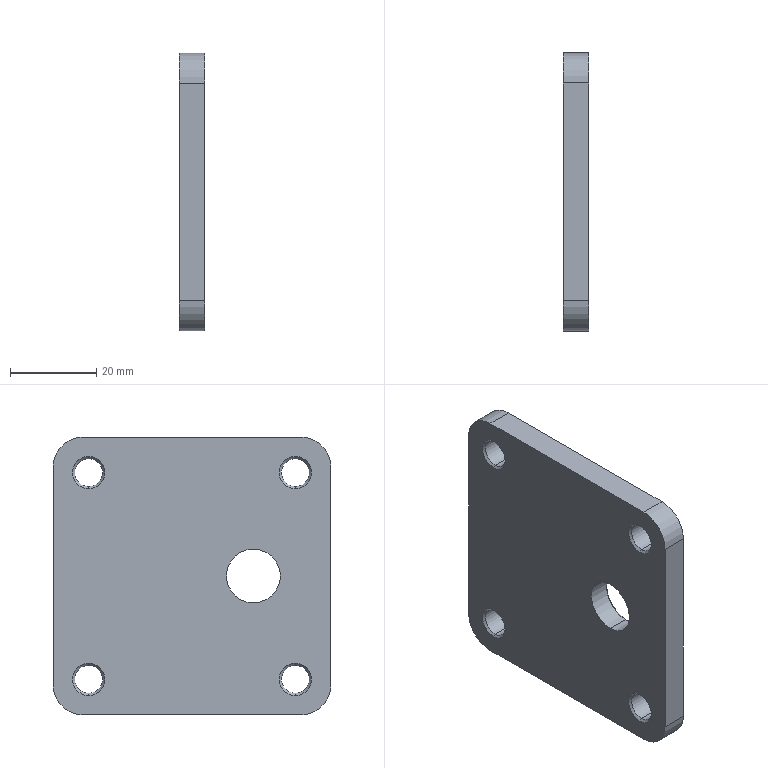Part | SolidWorks | features BaseBody 1 | 1 solid | 41 faces | box 6 x 64.5 x 64.5 mm | volume 23021 mm3 | cone 18 | cylinder 16 | plane 7 | commonest cylinder face diameters 6.5 x8 14 x4 12.5 x2 22 x2
STEP:
#1=CARTESIAN_POINT('',(443.9,24.75,6.25));
#2=VERTEX_POINT('',#1);
#3=CARTESIAN_POINT('',(443.9,24.75,-6.25));
#4=VERTEX_POINT('',#3);
#5=CARTESIAN_POINT('',(443.9,24.75,0.));
#6=DIRECTION('',(1.,0.,0.));
#7=DIRECTION('',(0.,0.,1.));
#8=AXIS2_PLACEMENT_3D('',#5,#6,#7);
#9=CIRCLE('',#8,6.25);
#10=EDGE_CURVE('',#2,#4,#9,.T.);
#11=ORIENTED_EDGE('',*,*,#10,.F.);
#12=CARTESIAN_POINT('',(444.4,24.75,6.75));
#13=VERTEX_POINT('',#12);
#14=CARTESIAN_POINT('',(443.9,24.75,6.25));
#15=DIRECTION('',(0.7071,0.,0.7071));
#16=VECTOR('',#15,1000.);
#17=LINE('',#14,#16);
#18=EDGE_CURVE('',#2,#13,#17,.T.);
#19=ORIENTED_EDGE('',*,*,#18,.T.);
#20=CARTESIAN_POINT('',(444.4,24.75,-6.75));
#21=VERTEX_POINT('',#20);
#22=CARTESIAN_POINT('',(444.4,24.75,0.));
#23=DIRECTION('',(-1.,0.,0.));
#24=DIRECTION('',(0.,0.,1.));
#25=AXIS2_PLACEMENT_3D('',#22,#23,#24);
#26=CIRCLE('',#25,6.75);
#27=EDGE_CURVE('',#21,#13,#26,.T.);
#28=ORIENTED_EDGE('',*,*,#27,.F.);
#29=CARTESIAN_POINT('',(443.9,24.75,-6.25));
#30=DIRECTION('',(0.7071,0.,-0.7071));
#31=VECTOR('',#30,1000.);
#32=LINE('',#29,#31);
#33=EDGE_CURVE('',#4,#21,#32,.T.);
#34=ORIENTED_EDGE('',*,*,#33,.F.);
#35=EDGE_LOOP('',(#11,#19,#28,#34));
#36=FACE_OUTER_BOUND('',#35,.T.);
#37=CARTESIAN_POINT('',(443.9,24.75,0.));
#38=DIRECTION('',(1.,0.,0.));
#39=DIRECTION('',(0.,0.,-1.));
#40=AXIS2_PLACEMENT_3D('',#37,#38,#39);
#41=CONICAL_SURFACE('',#40,6.25,0.7854);
#42=ADVANCED_FACE('',(#36),#41,.F.);
#43=CARTESIAN_POINT('',(444.4,63.,27.25));
#44=VERTEX_POINT('',#43);
#45=CARTESIAN_POINT('',(444.4,63.,20.75));
#46=VERTEX_POINT('',#45);
#47=CARTESIAN_POINT('',(444.4,63.,24.));
#48=DIRECTION('',(1.,0.,0.));
#49=DIRECTION('',(0.,0.,-1.));
#50=AXIS2_PLACEMENT_3D('',#47,#48,#49);
#51=CIRCLE('',#50,3.25);
#52=EDGE_CURVE('',#44,#46,#51,.T.);
#53=ORIENTED_EDGE('',*,*,#52,.F.);
#54=CARTESIAN_POINT('',(444.9,63.,27.75));
#55=VERTEX_POINT('',#54);
#56=CARTESIAN_POINT('',(444.4,63.,27.25));
#57=DIRECTION('',(0.7071,0.,0.7071));
#58=VECTOR('',#57,1000.);
#59=LINE('',#56,#58);
#60=EDGE_CURVE('',#44,#55,#59,.T.);
#61=ORIENTED_EDGE('',*,*,#60,.T.);
#62=CARTESIAN_POINT('',(444.9,63.,20.25));
#63=VERTEX_POINT('',#62);
#64=CARTESIAN_POINT('',(444.9,63.,24.));
#65=DIRECTION('',(-1.,0.,0.));
#66=DIRECTION('',(0.,0.,-1.));
#67=AXIS2_PLACEMENT_3D('',#64,#65,#66);
#68=CIRCLE('',#67,3.75);
#69=EDGE_CURVE('',#63,#55,#68,.T.);
#70=ORIENTED_EDGE('',*,*,#69,.F.);
#71=CARTESIAN_POINT('',(444.4,63.,20.75));
#72=DIRECTION('',(0.7071,0.,-0.7071));
#73=VECTOR('',#72,1000.);
#74=LINE('',#71,#73);
#75=EDGE_CURVE('',#46,#63,#74,.T.);
#76=ORIENTED_EDGE('',*,*,#75,.F.);
#77=EDGE_LOOP('',(#53,#61,#70,#76));
#78=FACE_OUTER_BOUND('',#77,.T.);
#79=CARTESIAN_POINT('',(444.4,63.,24.));
#80=DIRECTION('',(1.,0.,0.));
#81=DIRECTION('',(0.,0.,-1.));
#82=AXIS2_PLACEMENT_3D('',#79,#80,#81);
#83=CONICAL_SURFACE('',#82,3.25,0.7854);
#84=ADVANCED_FACE('',(#78),#83,.F.);
#85=CARTESIAN_POINT('',(444.4,63.,-20.75));
#86=VERTEX_POINT('',#85);
#87=CARTESIAN_POINT('',(444.4,63.,-27.25));
#88=VERTEX_POINT('',#87);
#89=CARTESIAN_POINT('',(444.4,63.,-24.));
#90=DIRECTION('',(1.,0.,0.));
#91=DIRECTION('',(0.,0.,-1.));
#92=AXIS2_PLACEMENT_3D('',#89,#90,#91);
#93=CIRCLE('',#92,3.25);
#94=EDGE_CURVE('',#86,#88,#93,.T.);
#95=ORIENTED_EDGE('',*,*,#94,.F.);
#96=CARTESIAN_POINT('',(444.9,63.,-20.25));
#97=VERTEX_POINT('',#96);
#98=CARTESIAN_POINT('',(444.4,63.,-20.75));
#99=DIRECTION('',(0.7071,0.,0.7071));
#100=VECTOR('',#99,1000.);
#101=LINE('',#98,#100);
#102=EDGE_CURVE('',#86,#97,#101,.T.);
#103=ORIENTED_EDGE('',*,*,#102,.T.);
#104=CARTESIAN_POINT('',(444.9,63.,-27.75));
#105=VERTEX_POINT('',#104);
#106=CARTESIAN_POINT('',(444.9,63.,-24.));
#107=DIRECTION('',(-1.,0.,0.));
#108=DIRECTION('',(0.,0.,-1.));
#109=AXIS2_PLACEMENT_3D('',#106,#107,#108);
#110=CIRCLE('',#109,3.75);
#111=EDGE_CURVE('',#105,#97,#110,.T.);
#112=ORIENTED_EDGE('',*,*,#111,.F.);
#113=CARTESIAN_POINT('',(444.4,63.,-27.25));
#114=DIRECTION('',(0.7071,0.,-0.7071));
#115=VECTOR('',#114,1000.);
#116=LINE('',#113,#115);
#117=EDGE_CURVE('',#88,#105,#116,.T.);
#118=ORIENTED_EDGE('',*,*,#117,.F.);
#119=EDGE_LOOP('',(#95,#103,#112,#118));
#120=FACE_OUTER_BOUND('',#119,.T.);
#121=CARTESIAN_POINT('',(444.4,63.,-24.));
#122=DIRECTION('',(1.,0.,0.));
#123=DIRECTION('',(0.,0.,-1.));
#124=AXIS2_PLACEMENT_3D('',#121,#122,#123);
#125=CONICAL_SURFACE('',#124,3.25,0.7854);
#126=ADVANCED_FACE('',(#120),#125,.F.);
#127=CARTESIAN_POINT('',(444.4,15.,-20.75));
#128=VERTEX_POINT('',#127);
#129=CARTESIAN_POINT('',(444.4,15.,-27.25));
#130=VERTEX_POINT('',#129);
#131=CARTESIAN_POINT('',(444.4,15.,-24.));
#132=DIRECTION('',(1.,0.,0.));
#133=DIRECTION('',(0.,0.,-1.));
#134=AXIS2_PLACEMENT_3D('',#131,#132,#133);
#135=CIRCLE('',#134,3.25);
#136=EDGE_CURVE('',#128,#130,#135,.T.);
#137=ORIENTED_EDGE('',*,*,#136,.F.);
#138=CARTESIAN_POINT('',(444.9,15.,-20.25));
#139=VERTEX_POINT('',#138);
#140=CARTESIAN_POINT('',(444.4,15.,-20.75));
#141=DIRECTION('',(0.7071,0.,0.7071));
#142=VECTOR('',#141,1000.);
#143=LINE('',#140,#142);
#144=EDGE_CURVE('',#128,#139,#143,.T.);
#145=ORIENTED_EDGE('',*,*,#144,.T.);
#146=CARTESIAN_POINT('',(444.9,15.,-27.75));
#147=VERTEX_POINT('',#146);
#148=CARTESIAN_POINT('',(444.9,15.,-24.));
#149=DIRECTION('',(-1.,0.,0.));
#150=DIRECTION('',(0.,0.,-1.));
#151=AXIS2_PLACEMENT_3D('',#148,#149,#150);
#152=CIRCLE('',#151,3.75);
#153=EDGE_CURVE('',#147,#139,#152,.T.);
#154=ORIENTED_EDGE('',*,*,#153,.F.);
#155=CARTESIAN_POINT('',(444.4,15.,-27.25));
#156=DIRECTION('',(0.7071,0.,-0.7071));
#157=VECTOR('',#156,1000.);
#158=LINE('',#155,#157);
#159=EDGE_CURVE('',#130,#147,#158,.T.);
#160=ORIENTED_EDGE('',*,*,#159,.F.);
#161=EDGE_LOOP('',(#137,#145,#154,#160));
#162=FACE_OUTER_BOUND('',#161,.T.);
#163=CARTESIAN_POINT('',(444.4,15.,-24.));
#164=DIRECTION('',(1.,0.,0.));
#165=DIRECTION('',(0.,0.,-1.));
#166=AXIS2_PLACEMENT_3D('',#163,#164,#165);
#167=CONICAL_SURFACE('',#166,3.25,0.7854);
#168=ADVANCED_FACE('',(#162),#167,.F.);
#169=CARTESIAN_POINT('',(444.4,15.,27.25));
#170=VERTEX_POINT('',#169);
#171=CARTESIAN_POINT('',(444.4,15.,20.75));
#172=VERTEX_POINT('',#171);
#173=CARTESIAN_POINT('',(444.4,15.,24.));
#174=DIRECTION('',(1.,0.,0.));
#175=DIRECTION('',(0.,0.,-1.));
#176=AXIS2_PLACEMENT_3D('',#173,#174,#175);
#177=CIRCLE('',#176,3.25);
#178=EDGE_CURVE('',#170,#172,#177,.T.);
#179=ORIENTED_EDGE('',*,*,#178,.F.);
#180=CARTESIAN_POINT('',(444.9,15.,27.75));
#181=VERTEX_POINT('',#180);
#182=CARTESIAN_POINT('',(444.4,15.,27.25));
#183=DIRECTION('',(0.7071,0.,0.7071));
#184=VECTOR('',#183,1000.);
#185=LINE('',#182,#184);
#186=EDGE_CURVE('',#170,#181,#185,.T.);
#187=ORIENTED_EDGE('',*,*,#186,.T.);
#188=CARTESIAN_POINT('',(444.9,15.,20.25));
#189=VERTEX_POINT('',#188);
#190=CARTESIAN_POINT('',(444.9,15.,24.));
#191=DIRECTION('',(-1.,0.,0.));
#192=DIRECTION('',(0.,0.,-1.));
#193=AXIS2_PLACEMENT_3D('',#190,#191,#192);
#194=CIRCLE('',#193,3.75);
#195=EDGE_CURVE('',#189,#181,#194,.T.);
#196=ORIENTED_EDGE('',*,*,#195,.F.);
#197=CARTESIAN_POINT('',(444.4,15.,20.75));
#198=DIRECTION('',(0.7071,0.,-0.7071));
#199=VECTOR('',#198,1000.);
#200=LINE('',#197,#199);
#201=EDGE_CURVE('',#172,#189,#200,.T.);
#202=ORIENTED_EDGE('',*,*,#201,.F.);
#203=EDGE_LOOP('',(#179,#187,#196,#202));
#204=FACE_OUTER_BOUND('',#203,.T.);
#205=CARTESIAN_POINT('',(444.4,15.,24.));
#206=DIRECTION('',(1.,0.,0.));
#207=DIRECTION('',(0.,0.,-1.));
#208=AXIS2_PLACEMENT_3D('',#205,#206,#207);
#209=CONICAL_SURFACE('',#208,3.25,0.7854);
#210=ADVANCED_FACE('',(#204),#209,.F.);
#211=CARTESIAN_POINT('',(439.4,63.,20.75));
#212=VERTEX_POINT('',#211);
#213=CARTESIAN_POINT('',(439.4,63.,27.25));
#214=VERTEX_POINT('',#213);
#215=CARTESIAN_POINT('',(439.4,63.,24.));
#216=DIRECTION('',(-1.,0.,0.));
#217=DIRECTION('',(0.,0.,-1.));
#218=AXIS2_PLACEMENT_3D('',#215,#216,#217);
#219=CIRCLE('',#218,3.25);
#220=EDGE_CURVE('',#212,#214,#219,.T.);
#221=ORIENTED_EDGE('',*,*,#220,.F.);
#222=CARTESIAN_POINT('',(438.9,63.,20.25));
#223=VERTEX_POINT('',#222);
#224=CARTESIAN_POINT('',(438.9,63.,20.25));
#225=DIRECTION('',(-0.7071,0.,-0.7071));
#226=VECTOR('',#225,1000.);
#227=LINE('',#224,#226);
#228=EDGE_CURVE('',#212,#223,#227,.T.);
#229=ORIENTED_EDGE('',*,*,#228,.T.);
#230=CARTESIAN_POINT('',(438.9,63.,27.75));
#231=VERTEX_POINT('',#230);
#232=CARTESIAN_POINT('',(438.9,63.,24.));
#233=DIRECTION('',(1.,0.,0.));
#234=DIRECTION('',(0.,0.,-1.));
#235=AXIS2_PLACEMENT_3D('',#232,#233,#234);
#236=CIRCLE('',#235,3.75);
#237=EDGE_CURVE('',#231,#223,#236,.T.);
#238=ORIENTED_EDGE('',*,*,#237,.F.);
#239=CARTESIAN_POINT('',(438.9,63.,27.75));
#240=DIRECTION('',(-0.7071,0.,0.7071));
#241=VECTOR('',#240,1000.);
#242=LINE('',#239,#241);
#243=EDGE_CURVE('',#214,#231,#242,.T.);
#244=ORIENTED_EDGE('',*,*,#243,.F.);
#245=EDGE_LOOP('',(#221,#229,#238,#244));
#246=FACE_OUTER_BOUND('',#245,.T.);
#247=CARTESIAN_POINT('',(438.9,63.,24.));
#248=DIRECTION('',(-1.,0.,0.));
#249=DIRECTION('',(0.,0.,1.));
#250=AXIS2_PLACEMENT_3D('',#247,#248,#249);
#251=CONICAL_SURFACE('',#250,3.75,0.7854);
#252=ADVANCED_FACE('',(#246),#251,.F.);
#253=CARTESIAN_POINT('',(439.4,15.,20.75));
#254=VERTEX_POINT('',#253);
#255=CARTESIAN_POINT('',(439.4,15.,27.25));
#256=VERTEX_POINT('',#255);
#257=CARTESIAN_POINT('',(439.4,15.,24.));
#258=DIRECTION('',(-1.,0.,0.));
#259=DIRECTION('',(0.,0.,-1.));
#260=AXIS2_PLACEMENT_3D('',#257,#258,#259);
#261=CIRCLE('',#260,3.25);
#262=EDGE_CURVE('',#254,#256,#261,.T.);
#263=ORIENTED_EDGE('',*,*,#262,.F.);
#264=CARTESIAN_POINT('',(438.9,15.,20.25));
#265=VERTEX_POINT('',#264);
#266=CARTESIAN_POINT('',(438.9,15.,20.25));
#267=DIRECTION('',(-0.7071,0.,-0.7071));
#268=VECTOR('',#267,1000.);
#269=LINE('',#266,#268);
#270=EDGE_CURVE('',#254,#265,#269,.T.);
#271=ORIENTED_EDGE('',*,*,#270,.T.);
#272=CARTESIAN_POINT('',(438.9,15.,27.75));
#273=VERTEX_POINT('',#272);
#274=CARTESIAN_POINT('',(438.9,15.,24.));
#275=DIRECTION('',(1.,0.,0.));
#276=DIRECTION('',(0.,0.,-1.));
#277=AXIS2_PLACEMENT_3D('',#274,#275,#276);
#278=CIRCLE('',#277,3.75);
#279=EDGE_CURVE('',#273,#265,#278,.T.);
#280=ORIENTED_EDGE('',*,*,#279,.F.);
#281=CARTESIAN_POINT('',(438.9,15.,27.75));
#282=DIRECTION('',(-0.7071,0.,0.7071));
#283=VECTOR('',#282,1000.);
#284=LINE('',#281,#283);
#285=EDGE_CURVE('',#256,#273,#284,.T.);
#286=ORIENTED_EDGE('',*,*,#285,.F.);
#287=EDGE_LOOP('',(#263,#271,#280,#286));
#288=FACE_OUTER_BOUND('',#287,.T.);
#289=CARTESIAN_POINT('',(438.9,15.,24.));
#290=DIRECTION('',(-1.,0.,0.));
#291=DIRECTION('',(0.,0.,1.));
#292=AXIS2_PLACEMENT_3D('',#289,#290,#291);
#293=CONICAL_SURFACE('',#292,3.75,0.7854);
#294=ADVANCED_FACE('',(#288),#293,.F.);
#295=CARTESIAN_POINT('',(439.4,15.,-27.25));
#296=VERTEX_POINT('',#295);
#297=CARTESIAN_POINT('',(439.4,15.,-20.75));
#298=VERTEX_POINT('',#297);
#299=CARTESIAN_POINT('',(439.4,15.,-24.));
#300=DIRECTION('',(-1.,0.,0.));
#301=DIRECTION('',(0.,0.,-1.));
#302=AXIS2_PLACEMENT_3D('',#299,#300,#301);
#303=CIRCLE('',#302,3.25);
#304=EDGE_CURVE('',#296,#298,#303,.T.);
#305=ORIENTED_EDGE('',*,*,#304,.F.);
#306=CARTESIAN_POINT('',(438.9,15.,-27.75));
#307=VERTEX_POINT('',#306);
#308=CARTESIAN_POINT('',(438.9,15.,-27.75));
#309=DIRECTION('',(-0.7071,0.,-0.7071));
#310=VECTOR('',#309,1000.);
#311=LINE('',#308,#310);
#312=EDGE_CURVE('',#296,#307,#311,.T.);
#313=ORIENTED_EDGE('',*,*,#312,.T.);
#314=CARTESIAN_POINT('',(438.9,15.,-20.25));
#315=VERTEX_POINT('',#314);
#316=CARTESIAN_POINT('',(438.9,15.,-24.));
#317=DIRECTION('',(1.,0.,0.));
#318=DIRECTION('',(0.,0.,-1.));
#319=AXIS2_PLACEMENT_3D('',#316,#317,#318);
#320=CIRCLE('',#319,3.75);
#321=EDGE_CURVE('',#315,#307,#320,.T.);
#322=ORIENTED_EDGE('',*,*,#321,.F.);
#323=CARTESIAN_POINT('',(438.9,15.,-20.25));
#324=DIRECTION('',(-0.7071,0.,0.7071));
#325=VECTOR('',#324,1000.);
#326=LINE('',#323,#325);
#327=EDGE_CURVE('',#298,#315,#326,.T.);
#328=ORIENTED_EDGE('',*,*,#327,.F.);
#329=EDGE_LOOP('',(#305,#313,#322,#328));
#330=FACE_OUTER_BOUND('',#329,.T.);
#331=CARTESIAN_POINT('',(438.9,15.,-24.));
#332=DIRECTION('',(-1.,0.,0.));
#333=DIRECTION('',(0.,0.,1.));
#334=AXIS2_PLACEMENT_3D('',#331,#332,#333);
#335=CONICAL_SURFACE('',#334,3.75,0.7854);
#336=ADVANCED_FACE('',(#330),#335,.F.);
#337=CARTESIAN_POINT('',(439.4,63.,-27.25));
#338=VERTEX_POINT('',#337);
#339=CARTESIAN_POINT('',(439.4,63.,-20.75));
#340=VERTEX_POINT('',#339);
#341=CARTESIAN_POINT('',(439.4,63.,-24.));
#342=DIRECTION('',(-1.,0.,0.));
#343=DIRECTION('',(0.,0.,-1.));
#344=AXIS2_PLACEMENT_3D('',#341,#342,#343);
#345=CIRCLE('',#344,3.25);
#346=EDGE_CURVE('',#338,#340,#345,.T.);
#347=ORIENTED_EDGE('',*,*,#346,.F.);
#348=CARTESIAN_POINT('',(438.9,63.,-27.75));
#349=VERTEX_POINT('',#348);
#350=CARTESIAN_POINT('',(438.9,63.,-27.75));
#351=DIRECTION('',(-0.7071,0.,-0.7071));
#352=VECTOR('',#351,1000.);
#353=LINE('',#350,#352);
#354=EDGE_CURVE('',#338,#349,#353,.T.);
#355=ORIENTED_EDGE('',*,*,#354,.T.);
#356=CARTESIAN_POINT('',(438.9,63.,-20.25));
#357=VERTEX_POINT('',#356);
#358=CARTESIAN_POINT('',(438.9,63.,-24.));
#359=DIRECTION('',(1.,0.,0.));
#360=DIRECTION('',(0.,0.,-1.));
#361=AXIS2_PLACEMENT_3D('',#358,#359,#360);
#362=CIRCLE('',#361,3.75);
#363=EDGE_CURVE('',#357,#349,#362,.T.);
#364=ORIENTED_EDGE('',*,*,#363,.F.);
#365=CARTESIAN_POINT('',(438.9,63.,-20.25));
#366=DIRECTION('',(-0.7071,0.,0.7071));
#367=VECTOR('',#366,1000.);
#368=LINE('',#365,#367);
#369=EDGE_CURVE('',#340,#357,#368,.T.);
#370=ORIENTED_EDGE('',*,*,#369,.F.);
#371=EDGE_LOOP('',(#347,#355,#364,#370));
#372=FACE_OUTER_BOUND('',#371,.T.);
#373=CARTESIAN_POINT('',(438.9,63.,-24.));
#374=DIRECTION('',(-1.,0.,0.));
#375=DIRECTION('',(0.,0.,1.));
#376=AXIS2_PLACEMENT_3D('',#373,#374,#375);
#377=CONICAL_SURFACE('',#376,3.75,0.7854);
#378=ADVANCED_FACE('',(#372),#377,.F.);
#379=CARTESIAN_POINT('',(444.4,24.75,-11.));
#380=VERTEX_POINT('',#379);
#381=CARTESIAN_POINT('',(444.4,24.75,11.));
#382=VERTEX_POINT('',#381);
#383=CARTESIAN_POINT('',(444.4,24.75,0.));
#384=DIRECTION('',(-1.,0.,0.));
#385=DIRECTION('',(0.,0.,1.));
#386=AXIS2_PLACEMENT_3D('',#383,#384,#385);
#387=CIRCLE('',#386,11.);
#388=EDGE_CURVE('',#380,#382,#387,.T.);
#389=ORIENTED_EDGE('',*,*,#388,.T.);
#390=CARTESIAN_POINT('',(444.9,24.75,11.));
#391=VERTEX_POINT('',#390);
#392=CARTESIAN_POINT('',(444.4,24.75,11.));
#393=DIRECTION('',(1.,0.,0.));
#394=VECTOR('',#393,1000.);
#395=LINE('',#392,#394);
#396=EDGE_CURVE('',#382,#391,#395,.T.);
#397=ORIENTED_EDGE('',*,*,#396,.T.);
#398=CARTESIAN_POINT('',(444.9,24.75,-11.));
#399=VERTEX_POINT('',#398);
#400=CARTESIAN_POINT('',(444.9,24.75,0.));
#401=DIRECTION('',(-1.,0.,0.));
#402=DIRECTION('',(0.,0.,1.));
#403=AXIS2_PLACEMENT_3D('',#400,#401,#402);
#404=CIRCLE('',#403,11.);
#405=EDGE_CURVE('',#399,#391,#404,.T.);
#406=ORIENTED_EDGE('',*,*,#405,.F.);
#407=CARTESIAN_POINT('',(444.4,24.75,-11.));
#408=DIRECTION('',(1.,0.,0.));
#409=VECTOR('',#408,1000.);
#410=LINE('',#407,#409);
#411=EDGE_CURVE('',#380,#399,#410,.T.);
#412=ORIENTED_EDGE('',*,*,#411,.F.);
#413=EDGE_LOOP('',(#389,#397,#406,#412));
#414=FACE_OUTER_BOUND('',#413,.T.);
#415=CARTESIAN_POINT('',(444.4,24.75,0.));
#416=DIRECTION('',(1.,0.,0.));
#417=DIRECTION('',(0.,0.,-1.));
#418=AXIS2_PLACEMENT_3D('',#415,#416,#417);
#419=CYLINDRICAL_SURFACE('',#418,11.);
#420=ADVANCED_FACE('',(#414),#419,.F.);
#421=ORIENTED_EDGE('',*,*,#10,.T.);
#422=CARTESIAN_POINT('',(438.9,24.75,-6.25));
#423=VERTEX_POINT('',#422);
#424=CARTESIAN_POINT('',(444.9,24.75,-6.25));
#425=DIRECTION('',(-1.,0.,0.));
#426=VECTOR('',#425,1000.);
#427=LINE('',#424,#426);
#428=EDGE_CURVE('',#4,#423,#427,.T.);
#429=ORIENTED_EDGE('',*,*,#428,.T.);
#430=CARTESIAN_POINT('',(438.9,24.75,6.25));
#431=VERTEX_POINT('',#430);
#432=CARTESIAN_POINT('',(438.9,24.75,0.));
#433=DIRECTION('',(-1.,0.,0.));
#434=DIRECTION('',(0.,0.,1.));
#435=AXIS2_PLACEMENT_3D('',#432,#433,#434);
#436=CIRCLE('',#435,6.25);
#437=EDGE_CURVE('',#423,#431,#436,.T.);
#438=ORIENTED_EDGE('',*,*,#437,.T.);
#439=CARTESIAN_POINT('',(444.9,24.75,6.25));
#440=DIRECTION('',(-1.,0.,0.));
#441=VECTOR('',#440,1000.);
#442=LINE('',#439,#441);
#443=EDGE_CURVE('',#2,#431,#442,.T.);
#444=ORIENTED_EDGE('',*,*,#443,.F.);
#445=EDGE_LOOP('',(#421,#429,#438,#444));
#446=FACE_OUTER_BOUND('',#445,.T.);
#447=CARTESIAN_POINT('',(444.9,24.75,0.));
#448=DIRECTION('',(-1.,0.,0.));
#449=DIRECTION('',(0.,0.,1.));
#450=AXIS2_PLACEMENT_3D('',#447,#448,#449);
#451=CYLINDRICAL_SURFACE('',#450,6.25);
#452=ADVANCED_FACE('',(#446),#451,.F.);
#453=ORIENTED_EDGE('',*,*,#94,.T.);
#454=CARTESIAN_POINT('',(444.9,63.,-27.25));
#455=DIRECTION('',(-1.,0.,0.));
#456=VECTOR('',#455,1000.);
#457=LINE('',#454,#456);
#458=EDGE_CURVE('',#88,#338,#457,.T.);
#459=ORIENTED_EDGE('',*,*,#458,.T.);
#460=ORIENTED_EDGE('',*,*,#346,.T.);
#461=CARTESIAN_POINT('',(444.9,63.,-20.75));
#462=DIRECTION('',(-1.,0.,0.));
#463=VECTOR('',#462,1000.);
#464=LINE('',#461,#463);
#465=EDGE_CURVE('',#86,#340,#464,.T.);
#466=ORIENTED_EDGE('',*,*,#465,.F.);
#467=EDGE_LOOP('',(#453,#459,#460,#466));
#468=FACE_OUTER_BOUND('',#467,.T.);
#469=CARTESIAN_POINT('',(444.9,63.,-24.));
#470=DIRECTION('',(-1.,0.,0.));
#471=DIRECTION('',(0.,0.,1.));
#472=AXIS2_PLACEMENT_3D('',#469,#470,#471);
#473=CYLINDRICAL_SURFACE('',#472,3.25);
#474=ADVANCED_FACE('',(#468),#473,.F.);
#475=ORIENTED_EDGE('',*,*,#52,.T.);
#476=CARTESIAN_POINT('',(444.9,63.,20.75));
#477=DIRECTION('',(-1.,0.,0.));
#478=VECTOR('',#477,1000.);
#479=LINE('',#476,#478);
#480=EDGE_CURVE('',#46,#212,#479,.T.);
#481=ORIENTED_EDGE('',*,*,#480,.T.);
#482=ORIENTED_EDGE('',*,*,#220,.T.);
#483=CARTESIAN_POINT('',(444.9,63.,27.25));
#484=DIRECTION('',(-1.,0.,0.));
#485=VECTOR('',#484,1000.);
#486=LINE('',#483,#485);
#487=EDGE_CURVE('',#44,#214,#486,.T.);
#488=ORIENTED_EDGE('',*,*,#487,.F.);
#489=EDGE_LOOP('',(#475,#481,#482,#488));
#490=FACE_OUTER_BOUND('',#489,.T.);
#491=CARTESIAN_POINT('',(444.9,63.,24.));
#492=DIRECTION('',(-1.,0.,0.));
#493=DIRECTION('',(0.,0.,1.));
#494=AXIS2_PLACEMENT_3D('',#491,#492,#493);
#495=CYLINDRICAL_SURFACE('',#494,3.25);
#496=ADVANCED_FACE('',(#490),#495,.F.);
#497=ORIENTED_EDGE('',*,*,#136,.T.);
#498=CARTESIAN_POINT('',(444.9,15.,-27.25));
#499=DIRECTION('',(-1.,0.,0.));
#500=VECTOR('',#499,1000.);
#501=LINE('',#498,#500);
#502=EDGE_CURVE('',#130,#296,#501,.T.);
#503=ORIENTED_EDGE('',*,*,#502,.T.);
#504=ORIENTED_EDGE('',*,*,#304,.T.);
#505=CARTESIAN_POINT('',(444.9,15.,-20.75));
#506=DIRECTION('',(-1.,0.,0.));
#507=VECTOR('',#506,1000.);
#508=LINE('',#505,#507);
#509=EDGE_CURVE('',#128,#298,#508,.T.);
#510=ORIENTED_EDGE('',*,*,#509,.F.);
#511=EDGE_LOOP('',(#497,#503,#504,#510));
#512=FACE_OUTER_BOUND('',#511,.T.);
#513=CARTESIAN_POINT('',(444.9,15.,-24.));
#514=DIRECTION('',(-1.,0.,0.));
#515=DIRECTION('',(0.,0.,1.));
#516=AXIS2_PLACEMENT_3D('',#513,#514,#515);
#517=CYLINDRICAL_SURFACE('',#516,3.25);
#518=ADVANCED_FACE('',(#512),#517,.F.);
#519=ORIENTED_EDGE('',*,*,#178,.T.);
#520=CARTESIAN_POINT('',(444.9,15.,20.75));
#521=DIRECTION('',(-1.,0.,0.));
#522=VECTOR('',#521,1000.);
#523=LINE('',#520,#522);
#524=EDGE_CURVE('',#172,#254,#523,.T.);
#525=ORIENTED_EDGE('',*,*,#524,.T.);
#526=ORIENTED_EDGE('',*,*,#262,.T.);
#527=CARTESIAN_POINT('',(444.9,15.,27.25));
#528=DIRECTION('',(-1.,0.,0.));
#529=VECTOR('',#528,1000.);
#530=LINE('',#527,#529);
#531=EDGE_CURVE('',#170,#256,#530,.T.);
#532=ORIENTED_EDGE('',*,*,#531,.F.);
#533=EDGE_LOOP('',(#519,#525,#526,#532));
#534=FACE_OUTER_BOUND('',#533,.T.);
#535=CARTESIAN_POINT('',(444.9,15.,24.));
#536=DIRECTION('',(-1.,0.,0.));
#537=DIRECTION('',(0.,0.,1.));
#538=AXIS2_PLACEMENT_3D('',#535,#536,#537);
#539=CYLINDRICAL_SURFACE('',#538,3.25);
#540=ADVANCED_FACE('',(#534),#539,.F.);
#541=ORIENTED_EDGE('',*,*,#195,.T.);
#542=CARTESIAN_POINT('',(444.9,15.,24.));
#543=DIRECTION('',(-1.,0.,0.));
#544=DIRECTION('',(0.,0.,-1.));
#545=AXIS2_PLACEMENT_3D('',#542,#543,#544);
#546=CIRCLE('',#545,3.75);
#547=EDGE_CURVE('',#181,#189,#546,.T.);
#548=ORIENTED_EDGE('',*,*,#547,.T.);
#549=EDGE_LOOP('',(#541,#548));
#550=FACE_BOUND('',#549,.T.);
#551=ORIENTED_EDGE('',*,*,#153,.T.);
#552=CARTESIAN_POINT('',(444.9,15.,-24.));
#553=DIRECTION('',(-1.,0.,0.));
#554=DIRECTION('',(0.,0.,-1.));
#555=AXIS2_PLACEMENT_3D('',#552,#553,#554);
#556=CIRCLE('',#555,3.75);
#557=EDGE_CURVE('',#139,#147,#556,.T.);
#558=ORIENTED_EDGE('',*,*,#557,.T.);
#559=EDGE_LOOP('',(#551,#558));
#560=FACE_BOUND('',#559,.T.);
#561=ORIENTED_EDGE('',*,*,#111,.T.);
#562=CARTESIAN_POINT('',(444.9,63.,-24.));
#563=DIRECTION('',(-1.,0.,0.));
#564=DIRECTION('',(0.,0.,-1.));
#565=AXIS2_PLACEMENT_3D('',#562,#563,#564);
#566=CIRCLE('',#565,3.75);
#567=EDGE_CURVE('',#97,#105,#566,.T.);
#568=ORIENTED_EDGE('',*,*,#567,.T.);
#569=EDGE_LOOP('',(#561,#568));
#570=FACE_BOUND('',#569,.T.);
#571=ORIENTED_EDGE('',*,*,#69,.T.);
#572=CARTESIAN_POINT('',(444.9,63.,24.));
#573=DIRECTION('',(-1.,0.,0.));
#574=DIRECTION('',(0.,0.,-1.));
#575=AXIS2_PLACEMENT_3D('',#572,#573,#574);
#576=CIRCLE('',#575,3.75);
#577=EDGE_CURVE('',#55,#63,#576,.T.);
#578=ORIENTED_EDGE('',*,*,#577,.T.);
#579=EDGE_LOOP('',(#571,#578));
#580=FACE_BOUND('',#579,.T.);
#581=CARTESIAN_POINT('',(444.9,13.75,32.25));
#582=VERTEX_POINT('',#581);
#583=CARTESIAN_POINT('',(444.9,6.75,25.25));
#584=VERTEX_POINT('',#583);
#585=CARTESIAN_POINT('',(444.9,13.75,25.25));
#586=DIRECTION('',(1.,0.,0.));
#587=DIRECTION('',(0.,0.,-1.));
#588=AXIS2_PLACEMENT_3D('',#585,#586,#587);
#589=CIRCLE('',#588,7.);
#590=EDGE_CURVE('',#582,#584,#589,.T.);
#591=ORIENTED_EDGE('',*,*,#590,.T.);
#592=CARTESIAN_POINT('',(444.9,6.75,-25.25));
#593=VERTEX_POINT('',#592);
#594=CARTESIAN_POINT('',(444.9,6.75,25.25));
#595=DIRECTION('',(0.,0.,-1.));
#596=VECTOR('',#595,1000.);
#597=LINE('',#594,#596);
#598=EDGE_CURVE('',#584,#593,#597,.T.);
#599=ORIENTED_EDGE('',*,*,#598,.T.);
#600=CARTESIAN_POINT('',(444.9,13.75,-32.25));
#601=VERTEX_POINT('',#600);
#602=CARTESIAN_POINT('',(444.9,13.75,-25.25));
#603=DIRECTION('',(1.,0.,0.));
#604=DIRECTION('',(0.,0.,-1.));
#605=AXIS2_PLACEMENT_3D('',#602,#603,#604);
#606=CIRCLE('',#605,7.);
#607=EDGE_CURVE('',#593,#601,#606,.T.);
#608=ORIENTED_EDGE('',*,*,#607,.T.);
#609=CARTESIAN_POINT('',(444.9,64.25,-32.25));
#610=VERTEX_POINT('',#609);
#611=CARTESIAN_POINT('',(444.9,64.25,-32.25));
#612=DIRECTION('',(0.,1.,0.));
#613=VECTOR('',#612,1000.);
#614=LINE('',#611,#613);
#615=EDGE_CURVE('',#601,#610,#614,.T.);
#616=ORIENTED_EDGE('',*,*,#615,.T.);
#617=CARTESIAN_POINT('',(444.9,71.25,-25.25));
#618=VERTEX_POINT('',#617);
#619=CARTESIAN_POINT('',(444.9,64.25,-25.25));
#620=DIRECTION('',(1.,0.,0.));
#621=DIRECTION('',(0.,0.,1.));
#622=AXIS2_PLACEMENT_3D('',#619,#620,#621);
#623=CIRCLE('',#622,7.);
#624=EDGE_CURVE('',#610,#618,#623,.T.);
#625=ORIENTED_EDGE('',*,*,#624,.T.);
#626=CARTESIAN_POINT('',(444.9,71.25,25.25));
#627=VERTEX_POINT('',#626);
#628=CARTESIAN_POINT('',(444.9,71.25,25.25));
#629=DIRECTION('',(0.,0.,1.));
#630=VECTOR('',#629,1000.);
#631=LINE('',#628,#630);
#632=EDGE_CURVE('',#618,#627,#631,.T.);
#633=ORIENTED_EDGE('',*,*,#632,.T.);
#634=CARTESIAN_POINT('',(444.9,64.25,32.25));
#635=VERTEX_POINT('',#634);
#636=CARTESIAN_POINT('',(444.9,64.25,25.25));
#637=DIRECTION('',(1.,0.,0.));
#638=DIRECTION('',(0.,0.,-1.));
#639=AXIS2_PLACEMENT_3D('',#636,#637,#638);
#640=CIRCLE('',#639,7.);
#641=EDGE_CURVE('',#627,#635,#640,.T.);
#642=ORIENTED_EDGE('',*,*,#641,.T.);
#643=CARTESIAN_POINT('',(444.9,64.25,32.25));
#644=DIRECTION('',(0.,-1.,0.));
#645=VECTOR('',#644,1000.);
#646=LINE('',#643,#645);
#647=EDGE_CURVE('',#635,#582,#646,.T.);
#648=ORIENTED_EDGE('',*,*,#647,.T.);
#649=EDGE_LOOP('',(#591,#599,#608,#616,#625,#633,#642,#648));
#650=FACE_OUTER_BOUND('',#649,.T.);
#651=ORIENTED_EDGE('',*,*,#405,.T.);
#652=CARTESIAN_POINT('',(444.9,24.75,0.));
#653=DIRECTION('',(-1.,0.,0.));
#654=DIRECTION('',(0.,0.,1.));
#655=AXIS2_PLACEMENT_3D('',#652,#653,#654);
#656=CIRCLE('',#655,11.);
#657=EDGE_CURVE('',#391,#399,#656,.T.);
#658=ORIENTED_EDGE('',*,*,#657,.T.);
#659=EDGE_LOOP('',(#651,#658));
#660=FACE_BOUND('',#659,.T.);
#661=CARTESIAN_POINT('',(444.9,13.75,25.25));
#662=DIRECTION('',(1.,0.,0.));
#663=DIRECTION('',(0.,0.,-1.));
#664=AXIS2_PLACEMENT_3D('',#661,#662,#663);
#665=PLANE('',#664);
#666=ADVANCED_FACE('',(#550,#560,#570,#580,#650,#660),#665,.T.);
#667=ORIENTED_EDGE('',*,*,#363,.T.);
#668=CARTESIAN_POINT('',(438.9,63.,-24.));
#669=DIRECTION('',(1.,0.,0.));
#670=DIRECTION('',(0.,0.,-1.));
#671=AXIS2_PLACEMENT_3D('',#668,#669,#670);
#672=CIRCLE('',#671,3.75);
#673=EDGE_CURVE('',#349,#357,#672,.T.);
#674=ORIENTED_EDGE('',*,*,#673,.T.);
#675=EDGE_LOOP('',(#667,#674));
#676=FACE_BOUND('',#675,.T.);
#677=ORIENTED_EDGE('',*,*,#321,.T.);
#678=CARTESIAN_POINT('',(438.9,15.,-24.));
#679=DIRECTION('',(1.,0.,0.));
#680=DIRECTION('',(0.,0.,-1.));
#681=AXIS2_PLACEMENT_3D('',#678,#679,#680);
#682=CIRCLE('',#681,3.75);
#683=EDGE_CURVE('',#307,#315,#682,.T.);
#684=ORIENTED_EDGE('',*,*,#683,.T.);
#685=EDGE_LOOP('',(#677,#684));
#686=FACE_BOUND('',#685,.T.);
#687=ORIENTED_EDGE('',*,*,#279,.T.);
#688=CARTESIAN_POINT('',(438.9,15.,24.));
#689=DIRECTION('',(1.,0.,0.));
#690=DIRECTION('',(0.,0.,-1.));
#691=AXIS2_PLACEMENT_3D('',#688,#689,#690);
#692=CIRCLE('',#691,3.75);
#693=EDGE_CURVE('',#265,#273,#692,.T.);
#694=ORIENTED_EDGE('',*,*,#693,.T.);
#695=EDGE_LOOP('',(#687,#694));
#696=FACE_BOUND('',#695,.T.);
#697=ORIENTED_EDGE('',*,*,#237,.T.);
#698=CARTESIAN_POINT('',(438.9,63.,24.));
#699=DIRECTION('',(1.,0.,0.));
#700=DIRECTION('',(0.,0.,-1.));
#701=AXIS2_PLACEMENT_3D('',#698,#699,#700);
#702=CIRCLE('',#701,3.75);
#703=EDGE_CURVE('',#223,#231,#702,.T.);
#704=ORIENTED_EDGE('',*,*,#703,.T.);
#705=EDGE_LOOP('',(#697,#704));
#706=FACE_BOUND('',#705,.T.);
#707=CARTESIAN_POINT('',(438.9,24.75,0.));
#708=DIRECTION('',(-1.,0.,0.));
#709=DIRECTION('',(0.,0.,1.));
#710=AXIS2_PLACEMENT_3D('',#707,#708,#709);
#711=CIRCLE('',#710,6.25);
#712=EDGE_CURVE('',#431,#423,#711,.T.);
#713=ORIENTED_EDGE('',*,*,#712,.F.);
#714=ORIENTED_EDGE('',*,*,#437,.F.);
#715=EDGE_LOOP('',(#713,#714));
#716=FACE_BOUND('',#715,.T.);
#717=CARTESIAN_POINT('',(438.9,13.75,32.25));
#718=VERTEX_POINT('',#717);
#719=CARTESIAN_POINT('',(438.9,6.75,25.25));
#720=VERTEX_POINT('',#719);
#721=CARTESIAN_POINT('',(438.9,13.75,25.25));
#722=DIRECTION('',(1.,0.,0.));
#723=DIRECTION('',(0.,0.,-1.));
#724=AXIS2_PLACEMENT_3D('',#721,#722,#723);
#725=CIRCLE('',#724,7.);
#726=EDGE_CURVE('',#718,#720,#725,.T.);
#727=ORIENTED_EDGE('',*,*,#726,.F.);
#728=CARTESIAN_POINT('',(438.9,64.25,32.25));
#729=VERTEX_POINT('',#728);
#730=CARTESIAN_POINT('',(438.9,64.25,32.25));
#731=DIRECTION('',(0.,-1.,0.));
#732=VECTOR('',#731,1000.);
#733=LINE('',#730,#732);
#734=EDGE_CURVE('',#729,#718,#733,.T.);
#735=ORIENTED_EDGE('',*,*,#734,.F.);
#736=CARTESIAN_POINT('',(438.9,71.25,25.25));
#737=VERTEX_POINT('',#736);
#738=CARTESIAN_POINT('',(438.9,64.25,25.25));
#739=DIRECTION('',(1.,0.,0.));
#740=DIRECTION('',(0.,0.,-1.));
#741=AXIS2_PLACEMENT_3D('',#738,#739,#740);
#742=CIRCLE('',#741,7.);
#743=EDGE_CURVE('',#737,#729,#742,.T.);
#744=ORIENTED_EDGE('',*,*,#743,.F.);
#745=CARTESIAN_POINT('',(438.9,71.25,-25.25));
#746=VERTEX_POINT('',#745);
#747=CARTESIAN_POINT('',(438.9,71.25,25.25));
#748=DIRECTION('',(0.,0.,1.));
#749=VECTOR('',#748,1000.);
#750=LINE('',#747,#749);
#751=EDGE_CURVE('',#746,#737,#750,.T.);
#752=ORIENTED_EDGE('',*,*,#751,.F.);
#753=CARTESIAN_POINT('',(438.9,64.25,-32.25));
#754=VERTEX_POINT('',#753);
#755=CARTESIAN_POINT('',(438.9,64.25,-25.25));
#756=DIRECTION('',(1.,0.,0.));
#757=DIRECTION('',(0.,0.,1.));
#758=AXIS2_PLACEMENT_3D('',#755,#756,#757);
#759=CIRCLE('',#758,7.);
#760=EDGE_CURVE('',#754,#746,#759,.T.);
#761=ORIENTED_EDGE('',*,*,#760,.F.);
#762=CARTESIAN_POINT('',(438.9,13.75,-32.25));
#763=VERTEX_POINT('',#762);
#764=CARTESIAN_POINT('',(438.9,64.25,-32.25));
#765=DIRECTION('',(0.,1.,0.));
#766=VECTOR('',#765,1000.);
#767=LINE('',#764,#766);
#768=EDGE_CURVE('',#763,#754,#767,.T.);
#769=ORIENTED_EDGE('',*,*,#768,.F.);
#770=CARTESIAN_POINT('',(438.9,6.75,-25.25));
#771=VERTEX_POINT('',#770);
#772=CARTESIAN_POINT('',(438.9,13.75,-25.25));
#773=DIRECTION('',(1.,0.,0.));
#774=DIRECTION('',(0.,0.,-1.));
#775=AXIS2_PLACEMENT_3D('',#772,#773,#774);
#776=CIRCLE('',#775,7.);
#777=EDGE_CURVE('',#771,#763,#776,.T.);
#778=ORIENTED_EDGE('',*,*,#777,.F.);
#779=CARTESIAN_POINT('',(438.9,6.75,25.25));
#780=DIRECTION('',(0.,0.,-1.));
#781=VECTOR('',#780,1000.);
#782=LINE('',#779,#781);
#783=EDGE_CURVE('',#720,#771,#782,.T.);
#784=ORIENTED_EDGE('',*,*,#783,.F.);
#785=EDGE_LOOP('',(#727,#735,#744,#752,#761,#769,#778,#784));
#786=FACE_OUTER_BOUND('',#785,.T.);
#787=CARTESIAN_POINT('',(438.9,13.75,25.25));
#788=DIRECTION('',(1.,0.,0.));
#789=DIRECTION('',(0.,0.,-1.));
#790=AXIS2_PLACEMENT_3D('',#787,#788,#789);
#791=PLANE('',#790);
#792=ADVANCED_FACE('',(#676,#686,#696,#706,#716,#786),#791,.F.);
#793=ORIENTED_EDGE('',*,*,#726,.T.);
#794=CARTESIAN_POINT('',(444.9,6.75,25.25));
#795=DIRECTION('',(-1.,0.,0.));
#796=VECTOR('',#795,1000.);
#797=LINE('',#794,#796);
#798=EDGE_CURVE('',#584,#720,#797,.T.);
#799=ORIENTED_EDGE('',*,*,#798,.F.);
#800=ORIENTED_EDGE('',*,*,#590,.F.);
#801=CARTESIAN_POINT('',(444.9,13.75,32.25));
#802=DIRECTION('',(-1.,0.,0.));
#803=VECTOR('',#802,1000.);
#804=LINE('',#801,#803);
#805=EDGE_CURVE('',#582,#718,#804,.T.);
#806=ORIENTED_EDGE('',*,*,#805,.T.);
#807=EDGE_LOOP('',(#793,#799,#800,#806));
#808=FACE_OUTER_BOUND('',#807,.T.);
#809=CARTESIAN_POINT('',(444.9,13.75,25.25));
#810=DIRECTION('',(-1.,0.,0.));
#811=DIRECTION('',(0.,0.,1.));
#812=AXIS2_PLACEMENT_3D('',#809,#810,#811);
#813=CYLINDRICAL_SURFACE('',#812,7.);
#814=ADVANCED_FACE('',(#808),#813,.T.);
#815=ORIENTED_EDGE('',*,*,#783,.T.);
#816=CARTESIAN_POINT('',(444.9,6.75,-25.25));
#817=DIRECTION('',(-1.,0.,0.));
#818=VECTOR('',#817,1000.);
#819=LINE('',#816,#818);
#820=EDGE_CURVE('',#593,#771,#819,.T.);
#821=ORIENTED_EDGE('',*,*,#820,.F.);
#822=ORIENTED_EDGE('',*,*,#598,.F.);
#823=ORIENTED_EDGE('',*,*,#798,.T.);
#824=EDGE_LOOP('',(#815,#821,#822,#823));
#825=FACE_OUTER_BOUND('',#824,.T.);
#826=CARTESIAN_POINT('',(444.9,6.75,25.25));
#827=DIRECTION('',(0.,1.,0.));
#828=DIRECTION('',(1.,0.,0.));
#829=AXIS2_PLACEMENT_3D('',#826,#827,#828);
#830=PLANE('',#829);
#831=ADVANCED_FACE('',(#825),#830,.F.);
#832=ORIENTED_EDGE('',*,*,#777,.T.);
#833=CARTESIAN_POINT('',(444.9,13.75,-32.25));
#834=DIRECTION('',(-1.,0.,0.));
#835=VECTOR('',#834,1000.);
#836=LINE('',#833,#835);
#837=EDGE_CURVE('',#601,#763,#836,.T.);
#838=ORIENTED_EDGE('',*,*,#837,.F.);
#839=ORIENTED_EDGE('',*,*,#607,.F.);
#840=ORIENTED_EDGE('',*,*,#820,.T.);
#841=EDGE_LOOP('',(#832,#838,#839,#840));
#842=FACE_OUTER_BOUND('',#841,.T.);
#843=CARTESIAN_POINT('',(444.9,13.75,-25.25));
#844=DIRECTION('',(-1.,0.,0.));
#845=DIRECTION('',(0.,0.,1.));
#846=AXIS2_PLACEMENT_3D('',#843,#844,#845);
#847=CYLINDRICAL_SURFACE('',#846,7.);
#848=ADVANCED_FACE('',(#842),#847,.T.);
#849=ORIENTED_EDGE('',*,*,#768,.T.);
#850=CARTESIAN_POINT('',(444.9,64.25,-32.25));
#851=DIRECTION('',(-1.,0.,0.));
#852=VECTOR('',#851,1000.);
#853=LINE('',#850,#852);
#854=EDGE_CURVE('',#610,#754,#853,.T.);
#855=ORIENTED_EDGE('',*,*,#854,.F.);
#856=ORIENTED_EDGE('',*,*,#615,.F.);
#857=ORIENTED_EDGE('',*,*,#837,.T.);
#858=EDGE_LOOP('',(#849,#855,#856,#857));
#859=FACE_OUTER_BOUND('',#858,.T.);
#860=CARTESIAN_POINT('',(444.9,64.25,-32.25));
#861=DIRECTION('',(0.,0.,1.));
#862=DIRECTION('',(0.,-1.,0.));
#863=AXIS2_PLACEMENT_3D('',#860,#861,#862);
#864=PLANE('',#863);
#865=ADVANCED_FACE('',(#859),#864,.F.);
#866=ORIENTED_EDGE('',*,*,#760,.T.);
#867=CARTESIAN_POINT('',(444.9,71.25,-25.25));
#868=DIRECTION('',(-1.,0.,0.));
#869=VECTOR('',#868,1000.);
#870=LINE('',#867,#869);
#871=EDGE_CURVE('',#618,#746,#870,.T.);
#872=ORIENTED_EDGE('',*,*,#871,.F.);
#873=ORIENTED_EDGE('',*,*,#624,.F.);
#874=ORIENTED_EDGE('',*,*,#854,.T.);
#875=EDGE_LOOP('',(#866,#872,#873,#874));
#876=FACE_OUTER_BOUND('',#875,.T.);
#877=CARTESIAN_POINT('',(444.9,64.25,-25.25));
#878=DIRECTION('',(-1.,0.,0.));
#879=DIRECTION('',(0.,0.,1.));
#880=AXIS2_PLACEMENT_3D('',#877,#878,#879);
#881=CYLINDRICAL_SURFACE('',#880,7.);
#882=ADVANCED_FACE('',(#876),#881,.T.);
#883=ORIENTED_EDGE('',*,*,#751,.T.);
#884=CARTESIAN_POINT('',(444.9,71.25,25.25));
#885=DIRECTION('',(-1.,0.,0.));
#886=VECTOR('',#885,1000.);
#887=LINE('',#884,#886);
#888=EDGE_CURVE('',#627,#737,#887,.T.);
#889=ORIENTED_EDGE('',*,*,#888,.F.);
#890=ORIENTED_EDGE('',*,*,#632,.F.);
#891=ORIENTED_EDGE('',*,*,#871,.T.);
#892=EDGE_LOOP('',(#883,#889,#890,#891));
#893=FACE_OUTER_BOUND('',#892,.T.);
#894=CARTESIAN_POINT('',(444.9,71.25,25.25));
#895=DIRECTION('',(0.,-1.,0.));
#896=DIRECTION('',(-1.,0.,0.));
#897=AXIS2_PLACEMENT_3D('',#894,#895,#896);
#898=PLANE('',#897);
#899=ADVANCED_FACE('',(#893),#898,.F.);
#900=ORIENTED_EDGE('',*,*,#743,.T.);
#901=CARTESIAN_POINT('',(444.9,64.25,32.25));
#902=DIRECTION('',(-1.,0.,0.));
#903=VECTOR('',#902,1000.);
#904=LINE('',#901,#903);
#905=EDGE_CURVE('',#635,#729,#904,.T.);
#906=ORIENTED_EDGE('',*,*,#905,.F.);
#907=ORIENTED_EDGE('',*,*,#641,.F.);
#908=ORIENTED_EDGE('',*,*,#888,.T.);
#909=EDGE_LOOP('',(#900,#906,#907,#908));
#910=FACE_OUTER_BOUND('',#909,.T.);
#911=CARTESIAN_POINT('',(444.9,64.25,25.25));
#912=DIRECTION('',(-1.,0.,0.));
#913=DIRECTION('',(0.,0.,1.));
#914=AXIS2_PLACEMENT_3D('',#911,#912,#913);
#915=CYLINDRICAL_SURFACE('',#914,7.);
#916=ADVANCED_FACE('',(#910),#915,.T.);
#917=ORIENTED_EDGE('',*,*,#734,.T.);
#918=ORIENTED_EDGE('',*,*,#805,.F.);
#919=ORIENTED_EDGE('',*,*,#647,.F.);
#920=ORIENTED_EDGE('',*,*,#905,.T.);
#921=EDGE_LOOP('',(#917,#918,#919,#920));
#922=FACE_OUTER_BOUND('',#921,.T.);
#923=CARTESIAN_POINT('',(444.9,64.25,32.25));
#924=DIRECTION('',(0.,0.,-1.));
#925=DIRECTION('',(0.,1.,0.));
#926=AXIS2_PLACEMENT_3D('',#923,#924,#925);
#927=PLANE('',#926);
#928=ADVANCED_FACE('',(#922),#927,.F.);
#929=ORIENTED_EDGE('',*,*,#524,.F.);
#930=CARTESIAN_POINT('',(444.4,15.,24.));
#931=DIRECTION('',(1.,0.,0.));
#932=DIRECTION('',(0.,0.,-1.));
#933=AXIS2_PLACEMENT_3D('',#930,#931,#932);
#934=CIRCLE('',#933,3.25);
#935=EDGE_CURVE('',#172,#170,#934,.T.);
#936=ORIENTED_EDGE('',*,*,#935,.T.);
#937=ORIENTED_EDGE('',*,*,#531,.T.);
#938=CARTESIAN_POINT('',(439.4,15.,24.));
#939=DIRECTION('',(-1.,0.,0.));
#940=DIRECTION('',(0.,0.,-1.));
#941=AXIS2_PLACEMENT_3D('',#938,#939,#940);
#942=CIRCLE('',#941,3.25);
#943=EDGE_CURVE('',#256,#254,#942,.T.);
#944=ORIENTED_EDGE('',*,*,#943,.T.);
#945=EDGE_LOOP('',(#929,#936,#937,#944));
#946=FACE_OUTER_BOUND('',#945,.T.);
#947=CARTESIAN_POINT('',(444.9,15.,24.));
#948=DIRECTION('',(-1.,0.,0.));
#949=DIRECTION('',(0.,0.,1.));
#950=AXIS2_PLACEMENT_3D('',#947,#948,#949);
#951=CYLINDRICAL_SURFACE('',#950,3.25);
#952=ADVANCED_FACE('',(#946),#951,.F.);
#953=ORIENTED_EDGE('',*,*,#502,.F.);
#954=CARTESIAN_POINT('',(444.4,15.,-24.));
#955=DIRECTION('',(1.,0.,0.));
#956=DIRECTION('',(0.,0.,-1.));
#957=AXIS2_PLACEMENT_3D('',#954,#955,#956);
#958=CIRCLE('',#957,3.25);
#959=EDGE_CURVE('',#130,#128,#958,.T.);
#960=ORIENTED_EDGE('',*,*,#959,.T.);
#961=ORIENTED_EDGE('',*,*,#509,.T.);
#962=CARTESIAN_POINT('',(439.4,15.,-24.));
#963=DIRECTION('',(-1.,0.,0.));
#964=DIRECTION('',(0.,0.,-1.));
#965=AXIS2_PLACEMENT_3D('',#962,#963,#964);
#966=CIRCLE('',#965,3.25);
#967=EDGE_CURVE('',#298,#296,#966,.T.);
#968=ORIENTED_EDGE('',*,*,#967,.T.);
#969=EDGE_LOOP('',(#953,#960,#961,#968));
#970=FACE_OUTER_BOUND('',#969,.T.);
#971=CARTESIAN_POINT('',(444.9,15.,-24.));
#972=DIRECTION('',(-1.,0.,0.));
#973=DIRECTION('',(0.,0.,1.));
#974=AXIS2_PLACEMENT_3D('',#971,#972,#973);
#975=CYLINDRICAL_SURFACE('',#974,3.25);
#976=ADVANCED_FACE('',(#970),#975,.F.);
#977=ORIENTED_EDGE('',*,*,#480,.F.);
#978=CARTESIAN_POINT('',(444.4,63.,24.));
#979=DIRECTION('',(1.,0.,0.));
#980=DIRECTION('',(0.,0.,-1.));
#981=AXIS2_PLACEMENT_3D('',#978,#979,#980);
#982=CIRCLE('',#981,3.25);
#983=EDGE_CURVE('',#46,#44,#982,.T.);
#984=ORIENTED_EDGE('',*,*,#983,.T.);
#985=ORIENTED_EDGE('',*,*,#487,.T.);
#986=CARTESIAN_POINT('',(439.4,63.,24.));
#987=DIRECTION('',(-1.,0.,0.));
#988=DIRECTION('',(0.,0.,-1.));
#989=AXIS2_PLACEMENT_3D('',#986,#987,#988);
#990=CIRCLE('',#989,3.25);
#991=EDGE_CURVE('',#214,#212,#990,.T.);
#992=ORIENTED_EDGE('',*,*,#991,.T.);
#993=EDGE_LOOP('',(#977,#984,#985,#992));
#994=FACE_OUTER_BOUND('',#993,.T.);
#995=CARTESIAN_POINT('',(444.9,63.,24.));
#996=DIRECTION('',(-1.,0.,0.));
#997=DIRECTION('',(0.,0.,1.));
#998=AXIS2_PLACEMENT_3D('',#995,#996,#997);
#999=CYLINDRICAL_SURFACE('',#998,3.25);
#1000=ADVANCED_FACE('',(#994),#999,.F.);
#1001=ORIENTED_EDGE('',*,*,#458,.F.);
#1002=CARTESIAN_POINT('',(444.4,63.,-24.));
#1003=DIRECTION('',(1.,0.,0.));
#1004=DIRECTION('',(0.,0.,-1.));
#1005=AXIS2_PLACEMENT_3D('',#1002,#1003,#1004);
#1006=CIRCLE('',#1005,3.25);
#1007=EDGE_CURVE('',#88,#86,#1006,.T.);
#1008=ORIENTED_EDGE('',*,*,#1007,.T.);
#1009=ORIENTED_EDGE('',*,*,#465,.T.);
#1010=CARTESIAN_POINT('',(439.4,63.,-24.));
#1011=DIRECTION('',(-1.,0.,0.));
#1012=DIRECTION('',(0.,0.,-1.));
#1013=AXIS2_PLACEMENT_3D('',#1010,#1011,#1012);
#1014=CIRCLE('',#1013,3.25);
#1015=EDGE_CURVE('',#340,#338,#1014,.T.);
#1016=ORIENTED_EDGE('',*,*,#1015,.T.);
#1017=EDGE_LOOP('',(#1001,#1008,#1009,#1016));
#1018=FACE_OUTER_BOUND('',#1017,.T.);
#1019=CARTESIAN_POINT('',(444.9,63.,-24.));
#1020=DIRECTION('',(-1.,0.,0.));
#1021=DIRECTION('',(0.,0.,1.));
#1022=AXIS2_PLACEMENT_3D('',#1019,#1020,#1021);
#1023=CYLINDRICAL_SURFACE('',#1022,3.25);
#1024=ADVANCED_FACE('',(#1018),#1023,.F.);
#1025=ORIENTED_EDGE('',*,*,#428,.F.);
#1026=CARTESIAN_POINT('',(443.9,24.75,0.));
#1027=DIRECTION('',(1.,0.,0.));
#1028=DIRECTION('',(0.,0.,1.));
#1029=AXIS2_PLACEMENT_3D('',#1026,#1027,#1028);
#1030=CIRCLE('',#1029,6.25);
#1031=EDGE_CURVE('',#4,#2,#1030,.T.);
#1032=ORIENTED_EDGE('',*,*,#1031,.T.);
#1033=ORIENTED_EDGE('',*,*,#443,.T.);
#1034=ORIENTED_EDGE('',*,*,#712,.T.);
#1035=EDGE_LOOP('',(#1025,#1032,#1033,#1034));
#1036=FACE_OUTER_BOUND('',#1035,.T.);
#1037=CARTESIAN_POINT('',(444.9,24.75,0.));
#1038=DIRECTION('',(-1.,0.,0.));
#1039=DIRECTION('',(0.,0.,1.));
#1040=AXIS2_PLACEMENT_3D('',#1037,#1038,#1039);
#1041=CYLINDRICAL_SURFACE('',#1040,6.25);
#1042=ADVANCED_FACE('',(#1036),#1041,.F.);
#1043=ORIENTED_EDGE('',*,*,#27,.T.);
#1044=CARTESIAN_POINT('',(444.4,24.75,0.));
#1045=DIRECTION('',(-1.,0.,0.));
#1046=DIRECTION('',(0.,0.,1.));
#1047=AXIS2_PLACEMENT_3D('',#1044,#1045,#1046);
#1048=CIRCLE('',#1047,6.75);
#1049=EDGE_CURVE('',#13,#21,#1048,.T.);
#1050=ORIENTED_EDGE('',*,*,#1049,.T.);
#1051=EDGE_LOOP('',(#1043,#1050));
#1052=FACE_BOUND('',#1051,.T.);
#1053=ORIENTED_EDGE('',*,*,#388,.F.);
#1054=CARTESIAN_POINT('',(444.4,24.75,0.));
#1055=DIRECTION('',(-1.,0.,0.));
#1056=DIRECTION('',(0.,0.,1.));
#1057=AXIS2_PLACEMENT_3D('',#1054,#1055,#1056);
#1058=CIRCLE('',#1057,11.);
#1059=EDGE_CURVE('',#382,#380,#1058,.T.);
#1060=ORIENTED_EDGE('',*,*,#1059,.F.);
#1061=EDGE_LOOP('',(#1053,#1060));
#1062=FACE_OUTER_BOUND('',#1061,.T.);
#1063=CARTESIAN_POINT('',(444.4,24.75,0.));
#1064=DIRECTION('',(-1.,0.,0.));
#1065=DIRECTION('',(0.,0.,1.));
#1066=AXIS2_PLACEMENT_3D('',#1063,#1064,#1065);
#1067=PLANE('',#1066);
#1068=ADVANCED_FACE('',(#1052,#1062),#1067,.F.);
#1069=ORIENTED_EDGE('',*,*,#396,.F.);
#1070=ORIENTED_EDGE('',*,*,#1059,.T.);
#1071=ORIENTED_EDGE('',*,*,#411,.T.);
#1072=ORIENTED_EDGE('',*,*,#657,.F.);
#1073=EDGE_LOOP('',(#1069,#1070,#1071,#1072));
#1074=FACE_OUTER_BOUND('',#1073,.T.);
#1075=CARTESIAN_POINT('',(444.4,24.75,0.));
#1076=DIRECTION('',(1.,0.,0.));
#1077=DIRECTION('',(0.,0.,-1.));
#1078=AXIS2_PLACEMENT_3D('',#1075,#1076,#1077);
#1079=CYLINDRICAL_SURFACE('',#1078,11.);
#1080=ADVANCED_FACE('',(#1074),#1079,.F.);
#1081=ORIENTED_EDGE('',*,*,#354,.F.);
#1082=ORIENTED_EDGE('',*,*,#1015,.F.);
#1083=ORIENTED_EDGE('',*,*,#369,.T.);
#1084=ORIENTED_EDGE('',*,*,#673,.F.);
#1085=EDGE_LOOP('',(#1081,#1082,#1083,#1084));
#1086=FACE_OUTER_BOUND('',#1085,.T.);
#1087=CARTESIAN_POINT('',(438.9,63.,-24.));
#1088=DIRECTION('',(-1.,0.,0.));
#1089=DIRECTION('',(0.,0.,1.));
#1090=AXIS2_PLACEMENT_3D('',#1087,#1088,#1089);
#1091=CONICAL_SURFACE('',#1090,3.75,0.7854);
#1092=ADVANCED_FACE('',(#1086),#1091,.F.);
#1093=ORIENTED_EDGE('',*,*,#312,.F.);
#1094=ORIENTED_EDGE('',*,*,#967,.F.);
#1095=ORIENTED_EDGE('',*,*,#327,.T.);
#1096=ORIENTED_EDGE('',*,*,#683,.F.);
#1097=EDGE_LOOP('',(#1093,#1094,#1095,#1096));
#1098=FACE_OUTER_BOUND('',#1097,.T.);
#1099=CARTESIAN_POINT('',(438.9,15.,-24.));
#1100=DIRECTION('',(-1.,0.,0.));
#1101=DIRECTION('',(0.,0.,1.));
#1102=AXIS2_PLACEMENT_3D('',#1099,#1100,#1101);
#1103=CONICAL_SURFACE('',#1102,3.75,0.7854);
#1104=ADVANCED_FACE('',(#1098),#1103,.F.);
#1105=ORIENTED_EDGE('',*,*,#270,.F.);
#1106=ORIENTED_EDGE('',*,*,#943,.F.);
#1107=ORIENTED_EDGE('',*,*,#285,.T.);
#1108=ORIENTED_EDGE('',*,*,#693,.F.);
#1109=EDGE_LOOP('',(#1105,#1106,#1107,#1108));
#1110=FACE_OUTER_BOUND('',#1109,.T.);
#1111=CARTESIAN_POINT('',(438.9,15.,24.));
#1112=DIRECTION('',(-1.,0.,0.));
#1113=DIRECTION('',(0.,0.,1.));
#1114=AXIS2_PLACEMENT_3D('',#1111,#1112,#1113);
#1115=CONICAL_SURFACE('',#1114,3.75,0.7854);
#1116=ADVANCED_FACE('',(#1110),#1115,.F.);
#1117=ORIENTED_EDGE('',*,*,#228,.F.);
#1118=ORIENTED_EDGE('',*,*,#991,.F.);
#1119=ORIENTED_EDGE('',*,*,#243,.T.);
#1120=ORIENTED_EDGE('',*,*,#703,.F.);
#1121=EDGE_LOOP('',(#1117,#1118,#1119,#1120));
#1122=FACE_OUTER_BOUND('',#1121,.T.);
#1123=CARTESIAN_POINT('',(438.9,63.,24.));
#1124=DIRECTION('',(-1.,0.,0.));
#1125=DIRECTION('',(0.,0.,1.));
#1126=AXIS2_PLACEMENT_3D('',#1123,#1124,#1125);
#1127=CONICAL_SURFACE('',#1126,3.75,0.7854);
#1128=ADVANCED_FACE('',(#1122),#1127,.F.);
#1129=ORIENTED_EDGE('',*,*,#186,.F.);
#1130=ORIENTED_EDGE('',*,*,#935,.F.);
#1131=ORIENTED_EDGE('',*,*,#201,.T.);
#1132=ORIENTED_EDGE('',*,*,#547,.F.);
#1133=EDGE_LOOP('',(#1129,#1130,#1131,#1132));
#1134=FACE_OUTER_BOUND('',#1133,.T.);
#1135=CARTESIAN_POINT('',(444.4,15.,24.));
#1136=DIRECTION('',(1.,0.,0.));
#1137=DIRECTION('',(0.,0.,-1.));
#1138=AXIS2_PLACEMENT_3D('',#1135,#1136,#1137);
#1139=CONICAL_SURFACE('',#1138,3.25,0.7854);
#1140=ADVANCED_FACE('',(#1134),#1139,.F.);
#1141=ORIENTED_EDGE('',*,*,#144,.F.);
#1142=ORIENTED_EDGE('',*,*,#959,.F.);
#1143=ORIENTED_EDGE('',*,*,#159,.T.);
#1144=ORIENTED_EDGE('',*,*,#557,.F.);
#1145=EDGE_LOOP('',(#1141,#1142,#1143,#1144));
#1146=FACE_OUTER_BOUND('',#1145,.T.);
#1147=CARTESIAN_POINT('',(444.4,15.,-24.));
#1148=DIRECTION('',(1.,0.,0.));
#1149=DIRECTION('',(0.,0.,-1.));
#1150=AXIS2_PLACEMENT_3D('',#1147,#1148,#1149);
#1151=CONICAL_SURFACE('',#1150,3.25,0.7854);
#1152=ADVANCED_FACE('',(#1146),#1151,.F.);
#1153=ORIENTED_EDGE('',*,*,#102,.F.);
#1154=ORIENTED_EDGE('',*,*,#1007,.F.);
#1155=ORIENTED_EDGE('',*,*,#117,.T.);
#1156=ORIENTED_EDGE('',*,*,#567,.F.);
#1157=EDGE_LOOP('',(#1153,#1154,#1155,#1156));
#1158=FACE_OUTER_BOUND('',#1157,.T.);
#1159=CARTESIAN_POINT('',(444.4,63.,-24.));
#1160=DIRECTION('',(1.,0.,0.));
#1161=DIRECTION('',(0.,0.,-1.));
#1162=AXIS2_PLACEMENT_3D('',#1159,#1160,#1161);
#1163=CONICAL_SURFACE('',#1162,3.25,0.7854);
#1164=ADVANCED_FACE('',(#1158),#1163,.F.);
#1165=ORIENTED_EDGE('',*,*,#60,.F.);
#1166=ORIENTED_EDGE('',*,*,#983,.F.);
#1167=ORIENTED_EDGE('',*,*,#75,.T.);
#1168=ORIENTED_EDGE('',*,*,#577,.F.);
#1169=EDGE_LOOP('',(#1165,#1166,#1167,#1168));
#1170=FACE_OUTER_BOUND('',#1169,.T.);
#1171=CARTESIAN_POINT('',(444.4,63.,24.));
#1172=DIRECTION('',(1.,0.,0.));
#1173=DIRECTION('',(0.,0.,-1.));
#1174=AXIS2_PLACEMENT_3D('',#1171,#1172,#1173);
#1175=CONICAL_SURFACE('',#1174,3.25,0.7854);
#1176=ADVANCED_FACE('',(#1170),#1175,.F.);
#1177=ORIENTED_EDGE('',*,*,#18,.F.);
#1178=ORIENTED_EDGE('',*,*,#1031,.F.);
#1179=ORIENTED_EDGE('',*,*,#33,.T.);
#1180=ORIENTED_EDGE('',*,*,#1049,.F.);
#1181=EDGE_LOOP('',(#1177,#1178,#1179,#1180));
#1182=FACE_OUTER_BOUND('',#1181,.T.);
#1183=CARTESIAN_POINT('',(443.9,24.75,0.));
#1184=DIRECTION('',(1.,0.,0.));
#1185=DIRECTION('',(0.,0.,-1.));
#1186=AXIS2_PLACEMENT_3D('',#1183,#1184,#1185);
#1187=CONICAL_SURFACE('',#1186,6.25,0.7854);
#1188=ADVANCED_FACE('',(#1182),#1187,.F.);
#1189=CLOSED_SHELL('',(#42,#84,#126,#168,#210,#252,#294,#336,#378,#420,#452,#474,#496,#518,#540,#666,#792,#814,#831,#848,#865,#882,#899,#916,#928,#952,#976,#1000,#1024,#1042,#1068,#1080,#1092,#1104,#1116,#1128,#1140,#1152,#1164,#1176,#1188));
#1190=MANIFOLD_SOLID_BREP('',#1189);
#1191=CARTESIAN_POINT('',(0.,0.,0.));
#1192=DIRECTION('',(0.,0.,1.));
#1193=DIRECTION('',(1.,0.,0.));
#1194=AXIS2_PLACEMENT_3D('',#1191,#1192,#1193);
#1195=(LENGTH_UNIT()NAMED_UNIT(*)SI_UNIT(.MILLI.,.METRE.));
#1196=UNCERTAINTY_MEASURE_WITH_UNIT(LENGTH_MEASURE(0.00001),#1195,'','');
#1197=(NAMED_UNIT(*)PLANE_ANGLE_UNIT()SI_UNIT($,.RADIAN.));
#1198=(NAMED_UNIT(*)SI_UNIT($,.STERADIAN.)SOLID_ANGLE_UNIT());
#1199=(GEOMETRIC_REPRESENTATION_CONTEXT(3)GLOBAL_UNCERTAINTY_ASSIGNED_CONTEXT((#1196))GLOBAL_UNIT_ASSIGNED_CONTEXT((#1195,#1197,#1198))REPRESENTATION_CONTEXT('',''));
#1200=ADVANCED_BREP_SHAPE_REPRESENTATION('',(#1190,#1194),#1199);